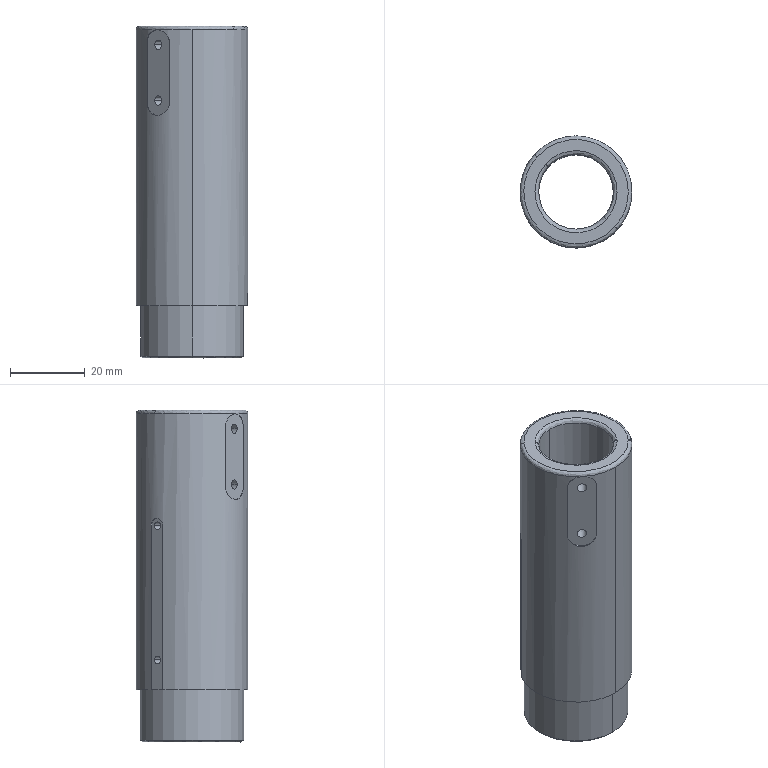Part | SolidWorks | features BaseBody 1 | 1 solid | 46 faces | box 30 x 30 x 89 mm | volume 33171 mm3 | cylinder 21 | plane 13 | spline 8 | cone 4 | commonest cylinder face diameters 2.05 x4 2.5 x4 5 x2 8 x2 20 x2 20.5 x2